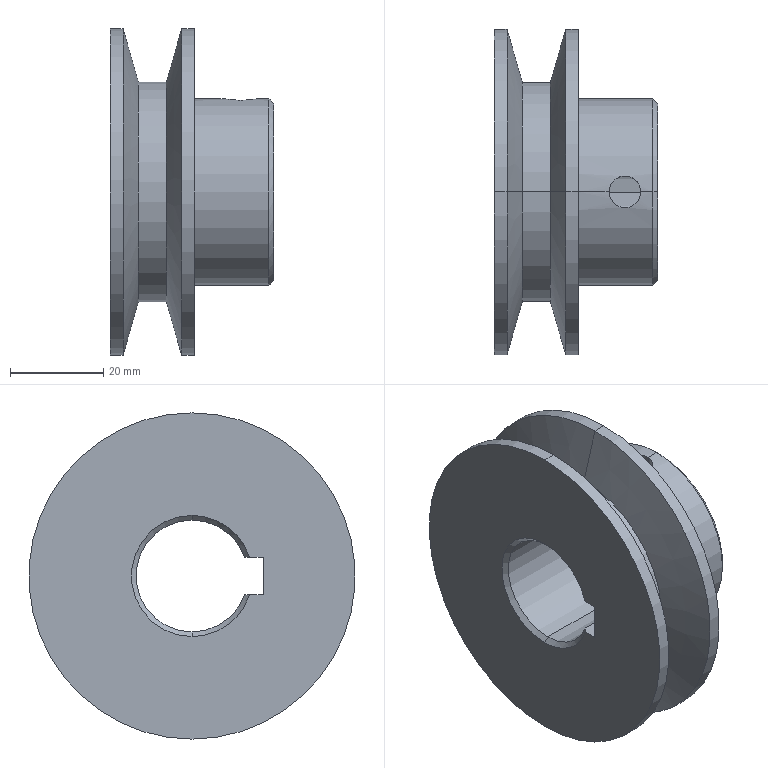Part | SolidWorks | features BaseBody 1 | 1 solid | 31 faces | box 35 x 70 x 70 mm | volume 53366 mm3 | cylinder 13 | cone 12 | plane 6 | commonest cylinder face diameters 70 x4 24 x3 6.8 x2 40 x2 47.1 x2
STEP:
#1=CARTESIAN_POINT('',(2.711,0.,35.));
#2=VERTEX_POINT('',#1);
#3=CARTESIAN_POINT('',(2.711,0.,-35.));
#4=VERTEX_POINT('',#3);
#5=CARTESIAN_POINT('',(2.711,0.,0.));
#6=DIRECTION('',(-1.,0.,0.));
#7=DIRECTION('',(0.,0.,1.));
#8=AXIS2_PLACEMENT_3D('',#5,#6,#7);
#9=CIRCLE('',#8,35.);
#10=EDGE_CURVE('',#2,#4,#9,.T.);
#11=ORIENTED_EDGE('',*,*,#10,.T.);
#12=CARTESIAN_POINT('',(0.,0.,-35.));
#13=VERTEX_POINT('',#12);
#14=CARTESIAN_POINT('',(0.,0.,-35.));
#15=DIRECTION('',(-1.,0.,0.));
#16=VECTOR('',#15,1000.);
#17=LINE('',#14,#16);
#18=EDGE_CURVE('',#4,#13,#17,.T.);
#19=ORIENTED_EDGE('',*,*,#18,.T.);
#20=CARTESIAN_POINT('',(0.,0.,35.));
#21=VERTEX_POINT('',#20);
#22=CARTESIAN_POINT('',(0.,0.,0.));
#23=DIRECTION('',(1.,0.,0.));
#24=DIRECTION('',(0.,0.,1.));
#25=AXIS2_PLACEMENT_3D('',#22,#23,#24);
#26=CIRCLE('',#25,35.);
#27=EDGE_CURVE('',#13,#21,#26,.T.);
#28=ORIENTED_EDGE('',*,*,#27,.T.);
#29=CARTESIAN_POINT('',(0.,0.,35.));
#30=DIRECTION('',(-1.,0.,0.));
#31=VECTOR('',#30,1000.);
#32=LINE('',#29,#31);
#33=EDGE_CURVE('',#2,#21,#32,.T.);
#34=ORIENTED_EDGE('',*,*,#33,.F.);
#35=EDGE_LOOP('',(#11,#19,#28,#34));
#36=FACE_OUTER_BOUND('',#35,.T.);
#37=CARTESIAN_POINT('',(0.,0.,0.));
#38=DIRECTION('',(-1.,0.,0.));
#39=DIRECTION('',(0.,0.,1.));
#40=AXIS2_PLACEMENT_3D('',#37,#38,#39);
#41=CYLINDRICAL_SURFACE('',#40,35.);
#42=ADVANCED_FACE('',(#36),#41,.T.);
#43=CARTESIAN_POINT('',(1.,0.,-12.));
#44=VERTEX_POINT('',#43);
#45=CARTESIAN_POINT('',(1.,-11.314,-4.));
#46=VERTEX_POINT('',#45);
#47=CARTESIAN_POINT('',(1.,0.,0.));
#48=DIRECTION('',(-1.,0.,0.));
#49=DIRECTION('',(0.,0.,1.));
#50=AXIS2_PLACEMENT_3D('',#47,#48,#49);
#51=CIRCLE('',#50,12.);
#52=EDGE_CURVE('',#44,#46,#51,.T.);
#53=ORIENTED_EDGE('',*,*,#52,.F.);
#54=CARTESIAN_POINT('',(0.,0.,-13.));
#55=VERTEX_POINT('',#54);
#56=CARTESIAN_POINT('',(0.,0.,-13.));
#57=DIRECTION('',(-0.7071,0.,-0.7071));
#58=VECTOR('',#57,1000.);
#59=LINE('',#56,#58);
#60=EDGE_CURVE('',#44,#55,#59,.T.);
#61=ORIENTED_EDGE('',*,*,#60,.T.);
#62=CARTESIAN_POINT('',(0.,-12.369,-4.));
#63=VERTEX_POINT('',#62);
#64=CARTESIAN_POINT('',(0.,0.,0.));
#65=DIRECTION('',(-1.,0.,0.));
#66=DIRECTION('',(0.,0.,1.));
#67=AXIS2_PLACEMENT_3D('',#64,#65,#66);
#68=CIRCLE('',#67,13.);
#69=EDGE_CURVE('',#55,#63,#68,.T.);
#70=ORIENTED_EDGE('',*,*,#69,.T.);
#71=CARTESIAN_POINT('',(1.,-11.314,-4.));
#72=CARTESIAN_POINT('',(0.6815,-11.652,-4.));
#73=CARTESIAN_POINT('',(0.3482,-12.003,-4.));
#74=CARTESIAN_POINT('',(0.,-12.369,-4.));
#75=B_SPLINE_CURVE_WITH_KNOTS('',3,(#71,#72,#73,#74),.UNSPECIFIED.,.F.,.F.,(4,4),(0.,1.),.UNSPECIFIED.);
#76=EDGE_CURVE('',#46,#63,#75,.T.);
#77=ORIENTED_EDGE('',*,*,#76,.F.);
#78=EDGE_LOOP('',(#53,#61,#70,#77));
#79=FACE_OUTER_BOUND('',#78,.T.);
#80=CARTESIAN_POINT('',(0.,0.,0.));
#81=DIRECTION('',(-1.,0.,0.));
#82=DIRECTION('',(0.,0.,1.));
#83=AXIS2_PLACEMENT_3D('',#80,#81,#82);
#84=CONICAL_SURFACE('',#83,13.,0.7854);
#85=ADVANCED_FACE('',(#79),#84,.F.);
#86=ORIENTED_EDGE('',*,*,#60,.F.);
#87=CARTESIAN_POINT('',(1.,0.,12.));
#88=VERTEX_POINT('',#87);
#89=CARTESIAN_POINT('',(1.,0.,0.));
#90=DIRECTION('',(-1.,0.,0.));
#91=DIRECTION('',(0.,0.,1.));
#92=AXIS2_PLACEMENT_3D('',#89,#90,#91);
#93=CIRCLE('',#92,12.);
#94=EDGE_CURVE('',#88,#44,#93,.T.);
#95=ORIENTED_EDGE('',*,*,#94,.F.);
#96=CARTESIAN_POINT('',(0.,0.,13.));
#97=VERTEX_POINT('',#96);
#98=CARTESIAN_POINT('',(0.,0.,13.));
#99=DIRECTION('',(-0.7071,0.,0.7071));
#100=VECTOR('',#99,1000.);
#101=LINE('',#98,#100);
#102=EDGE_CURVE('',#88,#97,#101,.T.);
#103=ORIENTED_EDGE('',*,*,#102,.T.);
#104=CARTESIAN_POINT('',(0.,0.,0.));
#105=DIRECTION('',(-1.,0.,0.));
#106=DIRECTION('',(0.,0.,1.));
#107=AXIS2_PLACEMENT_3D('',#104,#105,#106);
#108=CIRCLE('',#107,13.);
#109=EDGE_CURVE('',#97,#55,#108,.T.);
#110=ORIENTED_EDGE('',*,*,#109,.T.);
#111=EDGE_LOOP('',(#86,#95,#103,#110));
#112=FACE_OUTER_BOUND('',#111,.T.);
#113=CARTESIAN_POINT('',(0.,0.,0.));
#114=DIRECTION('',(-1.,0.,0.));
#115=DIRECTION('',(0.,0.,1.));
#116=AXIS2_PLACEMENT_3D('',#113,#114,#115);
#117=CONICAL_SURFACE('',#116,13.,0.7854);
#118=ADVANCED_FACE('',(#112),#117,.F.);
#119=CARTESIAN_POINT('',(5.995,0.,23.55));
#120=VERTEX_POINT('',#119);
#121=CARTESIAN_POINT('',(5.995,0.,-23.55));
#122=VERTEX_POINT('',#121);
#123=CARTESIAN_POINT('',(5.995,0.,0.));
#124=DIRECTION('',(-1.,0.,0.));
#125=DIRECTION('',(0.,0.,1.));
#126=AXIS2_PLACEMENT_3D('',#123,#124,#125);
#127=CIRCLE('',#126,23.55);
#128=EDGE_CURVE('',#120,#122,#127,.T.);
#129=ORIENTED_EDGE('',*,*,#128,.T.);
#130=CARTESIAN_POINT('',(2.711,0.,-35.));
#131=DIRECTION('',(-0.2756,0.,-0.9613));
#132=VECTOR('',#131,1000.);
#133=LINE('',#130,#132);
#134=EDGE_CURVE('',#122,#4,#133,.T.);
#135=ORIENTED_EDGE('',*,*,#134,.T.);
#136=ORIENTED_EDGE('',*,*,#10,.F.);
#137=CARTESIAN_POINT('',(2.711,0.,35.));
#138=DIRECTION('',(-0.2756,0.,0.9613));
#139=VECTOR('',#138,1000.);
#140=LINE('',#137,#139);
#141=EDGE_CURVE('',#120,#2,#140,.T.);
#142=ORIENTED_EDGE('',*,*,#141,.F.);
#143=EDGE_LOOP('',(#129,#135,#136,#142));
#144=FACE_OUTER_BOUND('',#143,.T.);
#145=CARTESIAN_POINT('',(2.711,0.,0.));
#146=DIRECTION('',(-1.,0.,0.));
#147=DIRECTION('',(0.,0.,1.));
#148=AXIS2_PLACEMENT_3D('',#145,#146,#147);
#149=CONICAL_SURFACE('',#148,35.,1.292);
#150=ADVANCED_FACE('',(#144),#149,.T.);
#151=CARTESIAN_POINT('',(34.,0.,-12.));
#152=VERTEX_POINT('',#151);
#153=CARTESIAN_POINT('',(34.,-11.314,-4.));
#154=VERTEX_POINT('',#153);
#155=CARTESIAN_POINT('',(34.,0.,0.));
#156=DIRECTION('',(-1.,0.,0.));
#157=DIRECTION('',(0.,0.,1.));
#158=AXIS2_PLACEMENT_3D('',#155,#156,#157);
#159=CIRCLE('',#158,12.);
#160=EDGE_CURVE('',#152,#154,#159,.T.);
#161=ORIENTED_EDGE('',*,*,#160,.F.);
#162=CARTESIAN_POINT('',(0.,0.,-12.));
#163=DIRECTION('',(-1.,0.,0.));
#164=VECTOR('',#163,1000.);
#165=LINE('',#162,#164);
#166=EDGE_CURVE('',#152,#44,#165,.T.);
#167=ORIENTED_EDGE('',*,*,#166,.T.);
#168=ORIENTED_EDGE('',*,*,#52,.T.);
#169=CARTESIAN_POINT('',(44.,-11.314,-4.));
#170=DIRECTION('',(1.,0.,0.));
#171=VECTOR('',#170,1000.);
#172=LINE('',#169,#171);
#173=EDGE_CURVE('',#46,#154,#172,.T.);
#174=ORIENTED_EDGE('',*,*,#173,.T.);
#175=EDGE_LOOP('',(#161,#167,#168,#174));
#176=FACE_OUTER_BOUND('',#175,.T.);
#177=CARTESIAN_POINT('',(0.,0.,0.));
#178=DIRECTION('',(-1.,0.,0.));
#179=DIRECTION('',(0.,0.,1.));
#180=AXIS2_PLACEMENT_3D('',#177,#178,#179);
#181=CYLINDRICAL_SURFACE('',#180,12.);
#182=ADVANCED_FACE('',(#176),#181,.F.);
#183=ORIENTED_EDGE('',*,*,#166,.F.);
#184=CARTESIAN_POINT('',(34.,0.,12.));
#185=VERTEX_POINT('',#184);
#186=CARTESIAN_POINT('',(34.,0.,0.));
#187=DIRECTION('',(-1.,0.,0.));
#188=DIRECTION('',(0.,0.,1.));
#189=AXIS2_PLACEMENT_3D('',#186,#187,#188);
#190=CIRCLE('',#189,12.);
#191=EDGE_CURVE('',#185,#152,#190,.T.);
#192=ORIENTED_EDGE('',*,*,#191,.F.);
#193=CARTESIAN_POINT('',(31.4,0.,12.));
#194=VERTEX_POINT('',#193);
#195=CARTESIAN_POINT('',(0.,0.,12.));
#196=DIRECTION('',(-1.,0.,0.));
#197=VECTOR('',#196,1000.);
#198=LINE('',#195,#197);
#199=EDGE_CURVE('',#185,#194,#198,.T.);
#200=ORIENTED_EDGE('',*,*,#199,.T.);
#201=CARTESIAN_POINT('',(24.6,0.,12.));
#202=VERTEX_POINT('',#201);
#203=CARTESIAN_POINT('',(24.6,0.,12.));
#204=CARTESIAN_POINT('',(24.6,0.2258,12.));
#205=CARTESIAN_POINT('',(24.622,0.4476,11.994));
#206=CARTESIAN_POINT('',(24.709,0.8837,11.969));
#207=CARTESIAN_POINT('',(24.775,1.1,11.951));
#208=CARTESIAN_POINT('',(24.946,1.511,11.906));
#209=CARTESIAN_POINT('',(25.051,1.706,11.88));
#210=CARTESIAN_POINT('',(25.297,2.075,11.821));
#211=CARTESIAN_POINT('',(25.44,2.248,11.789));
#212=CARTESIAN_POINT('',(25.752,2.56,11.725));
#213=CARTESIAN_POINT('',(25.922,2.701,11.693));
#214=CARTESIAN_POINT('',(26.293,2.949,11.633));
#215=CARTESIAN_POINT('',(26.489,3.054,11.605));
#216=CARTESIAN_POINT('',(26.898,3.224,11.559));
#217=CARTESIAN_POINT('',(27.113,3.29,11.54));
#218=CARTESIAN_POINT('',(27.552,3.378,11.515));
#219=CARTESIAN_POINT('',(27.774,3.4,11.508));
#220=CARTESIAN_POINT('',(28.22,3.4,11.508));
#221=CARTESIAN_POINT('',(28.446,3.378,11.515));
#222=CARTESIAN_POINT('',(28.883,3.291,11.54));
#223=CARTESIAN_POINT('',(29.096,3.226,11.558));
#224=CARTESIAN_POINT('',(29.509,3.055,11.605));
#225=CARTESIAN_POINT('',(29.706,2.949,11.633));
#226=CARTESIAN_POINT('',(30.073,2.704,11.692));
#227=CARTESIAN_POINT('',(30.246,2.562,11.724));
#228=CARTESIAN_POINT('',(30.56,2.248,11.789));
#229=CARTESIAN_POINT('',(30.7,2.078,11.82));
#230=CARTESIAN_POINT('',(30.946,1.711,11.879));
#231=CARTESIAN_POINT('',(31.053,1.512,11.906));
#232=CARTESIAN_POINT('',(31.224,1.102,11.951));
#233=CARTESIAN_POINT('',(31.289,0.8902,11.969));
#234=CARTESIAN_POINT('',(31.377,0.4517,11.994));
#235=CARTESIAN_POINT('',(31.4,0.2258,12.));
#236=CARTESIAN_POINT('',(31.4,0.,12.));
#237=B_SPLINE_CURVE_WITH_KNOTS('',3,(#203,#204,#205,#206,#207,#208,#209,#210,#211,#212,#213,#214,#215,#216,#217,#218,#219,#220,#221,#222,#223,#224,#225,#226,#227,#228,#229,#230,#231,#232,#233,#234,#235,#236),.UNSPECIFIED.,.F.,.F.,(4,2,2,2,2,2,2,2,2,2,2,2,2,2,2,2,4),(0.,0.0006676,0.001335,0.002003,0.00267,0.003338,0.004006,0.004673,0.005341,0.006008,0.006676,0.007343,0.008011,0.008679,0.009346,0.01001,0.01068),.UNSPECIFIED.);
#238=EDGE_CURVE('',#202,#194,#237,.T.);
#239=ORIENTED_EDGE('',*,*,#238,.F.);
#240=CARTESIAN_POINT('',(0.,0.,12.));
#241=DIRECTION('',(-1.,0.,0.));
#242=VECTOR('',#241,1000.);
#243=LINE('',#240,#242);
#244=EDGE_CURVE('',#202,#88,#243,.T.);
#245=ORIENTED_EDGE('',*,*,#244,.T.);
#246=ORIENTED_EDGE('',*,*,#94,.T.);
#247=EDGE_LOOP('',(#183,#192,#200,#239,#245,#246));
#248=FACE_OUTER_BOUND('',#247,.T.);
#249=CARTESIAN_POINT('',(0.,0.,0.));
#250=DIRECTION('',(-1.,0.,0.));
#251=DIRECTION('',(0.,0.,1.));
#252=AXIS2_PLACEMENT_3D('',#249,#250,#251);
#253=CYLINDRICAL_SURFACE('',#252,12.);
#254=ADVANCED_FACE('',(#248),#253,.F.);
#255=CARTESIAN_POINT('',(12.005,0.,23.55));
#256=VERTEX_POINT('',#255);
#257=CARTESIAN_POINT('',(12.005,0.,-23.55));
#258=VERTEX_POINT('',#257);
#259=CARTESIAN_POINT('',(12.005,0.,0.));
#260=DIRECTION('',(-1.,0.,0.));
#261=DIRECTION('',(0.,0.,1.));
#262=AXIS2_PLACEMENT_3D('',#259,#260,#261);
#263=CIRCLE('',#262,23.55);
#264=EDGE_CURVE('',#256,#258,#263,.T.);
#265=ORIENTED_EDGE('',*,*,#264,.T.);
#266=CARTESIAN_POINT('',(0.,0.,-23.55));
#267=DIRECTION('',(-1.,0.,0.));
#268=VECTOR('',#267,1000.);
#269=LINE('',#266,#268);
#270=EDGE_CURVE('',#258,#122,#269,.T.);
#271=ORIENTED_EDGE('',*,*,#270,.T.);
#272=ORIENTED_EDGE('',*,*,#128,.F.);
#273=CARTESIAN_POINT('',(0.,0.,23.55));
#274=DIRECTION('',(-1.,0.,0.));
#275=VECTOR('',#274,1000.);
#276=LINE('',#273,#275);
#277=EDGE_CURVE('',#256,#120,#276,.T.);
#278=ORIENTED_EDGE('',*,*,#277,.F.);
#279=EDGE_LOOP('',(#265,#271,#272,#278));
#280=FACE_OUTER_BOUND('',#279,.T.);
#281=CARTESIAN_POINT('',(0.,0.,0.));
#282=DIRECTION('',(-1.,0.,0.));
#283=DIRECTION('',(0.,0.,1.));
#284=AXIS2_PLACEMENT_3D('',#281,#282,#283);
#285=CYLINDRICAL_SURFACE('',#284,23.55);
#286=ADVANCED_FACE('',(#280),#285,.T.);
#287=CARTESIAN_POINT('',(34.,-11.314,4.));
#288=VERTEX_POINT('',#287);
#289=CARTESIAN_POINT('',(34.,0.,0.));
#290=DIRECTION('',(-1.,0.,0.));
#291=DIRECTION('',(0.,0.,1.));
#292=AXIS2_PLACEMENT_3D('',#289,#290,#291);
#293=CIRCLE('',#292,12.);
#294=EDGE_CURVE('',#288,#185,#293,.T.);
#295=ORIENTED_EDGE('',*,*,#294,.T.);
#296=CARTESIAN_POINT('',(35.,0.,13.));
#297=VERTEX_POINT('',#296);
#298=CARTESIAN_POINT('',(35.,0.,13.));
#299=DIRECTION('',(0.7071,0.,0.7071));
#300=VECTOR('',#299,1000.);
#301=LINE('',#298,#300);
#302=EDGE_CURVE('',#185,#297,#301,.T.);
#303=ORIENTED_EDGE('',*,*,#302,.T.);
#304=CARTESIAN_POINT('',(35.,-12.369,4.));
#305=VERTEX_POINT('',#304);
#306=CARTESIAN_POINT('',(35.,0.,0.));
#307=DIRECTION('',(1.,0.,0.));
#308=DIRECTION('',(0.,0.,-1.));
#309=AXIS2_PLACEMENT_3D('',#306,#307,#308);
#310=CIRCLE('',#309,13.);
#311=EDGE_CURVE('',#297,#305,#310,.T.);
#312=ORIENTED_EDGE('',*,*,#311,.T.);
#313=CARTESIAN_POINT('',(34.,-11.314,4.));
#314=CARTESIAN_POINT('',(34.318,-11.652,4.));
#315=CARTESIAN_POINT('',(34.652,-12.003,4.));
#316=CARTESIAN_POINT('',(35.,-12.369,4.));
#317=B_SPLINE_CURVE_WITH_KNOTS('',3,(#313,#314,#315,#316),.UNSPECIFIED.,.F.,.F.,(4,4),(0.,1.),.UNSPECIFIED.);
#318=EDGE_CURVE('',#288,#305,#317,.T.);
#319=ORIENTED_EDGE('',*,*,#318,.F.);
#320=EDGE_LOOP('',(#295,#303,#312,#319));
#321=FACE_OUTER_BOUND('',#320,.T.);
#322=CARTESIAN_POINT('',(35.,0.,0.));
#323=DIRECTION('',(1.,0.,0.));
#324=DIRECTION('',(0.,0.,-1.));
#325=AXIS2_PLACEMENT_3D('',#322,#323,#324);
#326=CONICAL_SURFACE('',#325,13.,0.7854);
#327=ADVANCED_FACE('',(#321),#326,.F.);
#328=ORIENTED_EDGE('',*,*,#302,.F.);
#329=ORIENTED_EDGE('',*,*,#191,.T.);
#330=CARTESIAN_POINT('',(35.,0.,-13.));
#331=VERTEX_POINT('',#330);
#332=CARTESIAN_POINT('',(35.,0.,-13.));
#333=DIRECTION('',(0.7071,0.,-0.7071));
#334=VECTOR('',#333,1000.);
#335=LINE('',#332,#334);
#336=EDGE_CURVE('',#152,#331,#335,.T.);
#337=ORIENTED_EDGE('',*,*,#336,.T.);
#338=CARTESIAN_POINT('',(35.,0.,0.));
#339=DIRECTION('',(1.,0.,0.));
#340=DIRECTION('',(0.,0.,-1.));
#341=AXIS2_PLACEMENT_3D('',#338,#339,#340);
#342=CIRCLE('',#341,13.);
#343=EDGE_CURVE('',#331,#297,#342,.T.);
#344=ORIENTED_EDGE('',*,*,#343,.T.);
#345=EDGE_LOOP('',(#328,#329,#337,#344));
#346=FACE_OUTER_BOUND('',#345,.T.);
#347=CARTESIAN_POINT('',(35.,0.,0.));
#348=DIRECTION('',(1.,0.,0.));
#349=DIRECTION('',(0.,0.,-1.));
#350=AXIS2_PLACEMENT_3D('',#347,#348,#349);
#351=CONICAL_SURFACE('',#350,13.,0.7854);
#352=ADVANCED_FACE('',(#346),#351,.F.);
#353=CARTESIAN_POINT('',(31.4,0.,20.));
#354=VERTEX_POINT('',#353);
#355=CARTESIAN_POINT('',(24.6,0.,20.));
#356=VERTEX_POINT('',#355);
#357=CARTESIAN_POINT('',(31.4,0.,20.));
#358=CARTESIAN_POINT('',(31.4,-0.225,20.));
#359=CARTESIAN_POINT('',(31.378,-0.4462,19.996));
#360=CARTESIAN_POINT('',(31.291,-0.8813,19.982));
#361=CARTESIAN_POINT('',(31.226,-1.097,19.971));
#362=CARTESIAN_POINT('',(31.055,-1.509,19.944));
#363=CARTESIAN_POINT('',(30.951,-1.704,19.928));
#364=CARTESIAN_POINT('',(30.704,-2.073,19.893));
#365=CARTESIAN_POINT('',(30.561,-2.248,19.874));
#366=CARTESIAN_POINT('',(30.248,-2.561,19.836));
#367=CARTESIAN_POINT('',(30.077,-2.701,19.817));
#368=CARTESIAN_POINT('',(29.705,-2.95,19.782));
#369=CARTESIAN_POINT('',(29.508,-3.055,19.765));
#370=CARTESIAN_POINT('',(29.099,-3.225,19.738));
#371=CARTESIAN_POINT('',(28.885,-3.291,19.728));
#372=CARTESIAN_POINT('',(28.446,-3.378,19.713));
#373=CARTESIAN_POINT('',(28.225,-3.4,19.709));
#374=CARTESIAN_POINT('',(27.78,-3.4,19.709));
#375=CARTESIAN_POINT('',(27.555,-3.378,19.713));
#376=CARTESIAN_POINT('',(27.118,-3.291,19.727));
#377=CARTESIAN_POINT('',(26.906,-3.227,19.738));
#378=CARTESIAN_POINT('',(26.494,-3.057,19.765));
#379=CARTESIAN_POINT('',(26.296,-2.95,19.782));
#380=CARTESIAN_POINT('',(25.928,-2.705,19.817));
#381=CARTESIAN_POINT('',(25.756,-2.564,19.836));
#382=CARTESIAN_POINT('',(25.439,-2.247,19.874));
#383=CARTESIAN_POINT('',(25.298,-2.076,19.893));
#384=CARTESIAN_POINT('',(25.052,-1.709,19.928));
#385=CARTESIAN_POINT('',(24.945,-1.51,19.944));
#386=CARTESIAN_POINT('',(24.775,-1.099,19.971));
#387=CARTESIAN_POINT('',(24.71,-0.8867,19.982));
#388=CARTESIAN_POINT('',(24.623,-0.4503,19.996));
#389=CARTESIAN_POINT('',(24.6,-0.225,20.));
#390=CARTESIAN_POINT('',(24.6,0.,20.));
#391=B_SPLINE_CURVE_WITH_KNOTS('',3,(#357,#358,#359,#360,#361,#362,#363,#364,#365,#366,#367,#368,#369,#370,#371,#372,#373,#374,#375,#376,#377,#378,#379,#380,#381,#382,#383,#384,#385,#386,#387,#388,#389,#390),.UNSPECIFIED.,.F.,.F.,(4,2,2,2,2,2,2,2,2,2,2,2,2,2,2,2,4),(0.01065,0.01131,0.01198,0.01264,0.01331,0.01397,0.01464,0.0153,0.01597,0.01664,0.0173,0.01797,0.01863,0.0193,0.01996,0.02063,0.02129),.UNSPECIFIED.);
#392=EDGE_CURVE('',#354,#356,#391,.T.);
#393=ORIENTED_EDGE('',*,*,#392,.F.);
#394=CARTESIAN_POINT('',(31.4,0.,0.));
#395=DIRECTION('',(0.,0.,-1.));
#396=VECTOR('',#395,1000.);
#397=LINE('',#394,#396);
#398=EDGE_CURVE('',#354,#194,#397,.T.);
#399=ORIENTED_EDGE('',*,*,#398,.T.);
#400=CARTESIAN_POINT('',(31.4,0.,12.));
#401=CARTESIAN_POINT('',(31.4,-0.2258,12.));
#402=CARTESIAN_POINT('',(31.378,-0.4476,11.994));
#403=CARTESIAN_POINT('',(31.291,-0.8837,11.969));
#404=CARTESIAN_POINT('',(31.225,-1.1,11.951));
#405=CARTESIAN_POINT('',(31.054,-1.511,11.906));
#406=CARTESIAN_POINT('',(30.949,-1.706,11.88));
#407=CARTESIAN_POINT('',(30.703,-2.075,11.821));
#408=CARTESIAN_POINT('',(30.56,-2.248,11.789));
#409=CARTESIAN_POINT('',(30.248,-2.56,11.725));
#410=CARTESIAN_POINT('',(30.078,-2.701,11.693));
#411=CARTESIAN_POINT('',(29.707,-2.949,11.633));
#412=CARTESIAN_POINT('',(29.511,-3.054,11.605));
#413=CARTESIAN_POINT('',(29.102,-3.224,11.559));
#414=CARTESIAN_POINT('',(28.887,-3.29,11.54));
#415=CARTESIAN_POINT('',(28.448,-3.378,11.515));
#416=CARTESIAN_POINT('',(28.226,-3.4,11.508));
#417=CARTESIAN_POINT('',(27.78,-3.4,11.508));
#418=CARTESIAN_POINT('',(27.554,-3.378,11.515));
#419=CARTESIAN_POINT('',(27.117,-3.291,11.54));
#420=CARTESIAN_POINT('',(26.904,-3.226,11.558));
#421=CARTESIAN_POINT('',(26.491,-3.055,11.605));
#422=CARTESIAN_POINT('',(26.294,-2.949,11.633));
#423=CARTESIAN_POINT('',(25.927,-2.704,11.692));
#424=CARTESIAN_POINT('',(25.754,-2.562,11.724));
#425=CARTESIAN_POINT('',(25.44,-2.248,11.789));
#426=CARTESIAN_POINT('',(25.3,-2.078,11.82));
#427=CARTESIAN_POINT('',(25.054,-1.711,11.879));
#428=CARTESIAN_POINT('',(24.947,-1.512,11.906));
#429=CARTESIAN_POINT('',(24.776,-1.102,11.951));
#430=CARTESIAN_POINT('',(24.711,-0.8902,11.969));
#431=CARTESIAN_POINT('',(24.623,-0.4517,11.994));
#432=CARTESIAN_POINT('',(24.6,-0.2258,12.));
#433=CARTESIAN_POINT('',(24.6,0.,12.));
#434=B_SPLINE_CURVE_WITH_KNOTS('',3,(#400,#401,#402,#403,#404,#405,#406,#407,#408,#409,#410,#411,#412,#413,#414,#415,#416,#417,#418,#419,#420,#421,#422,#423,#424,#425,#426,#427,#428,#429,#430,#431,#432,#433),.UNSPECIFIED.,.F.,.F.,(4,2,2,2,2,2,2,2,2,2,2,2,2,2,2,2,4),(0.01068,0.01135,0.01202,0.01268,0.01335,0.01402,0.01469,0.01535,0.01602,0.01669,0.01736,0.01802,0.01869,0.01936,0.02003,0.02069,0.02136),.UNSPECIFIED.);
#435=EDGE_CURVE('',#194,#202,#434,.T.);
#436=ORIENTED_EDGE('',*,*,#435,.T.);
#437=CARTESIAN_POINT('',(24.6,0.,0.));
#438=DIRECTION('',(0.,0.,-1.));
#439=VECTOR('',#438,1000.);
#440=LINE('',#437,#439);
#441=EDGE_CURVE('',#356,#202,#440,.T.);
#442=ORIENTED_EDGE('',*,*,#441,.F.);
#443=EDGE_LOOP('',(#393,#399,#436,#442));
#444=FACE_OUTER_BOUND('',#443,.T.);
#445=CARTESIAN_POINT('',(28.,0.,0.));
#446=DIRECTION('',(0.,0.,-1.));
#447=DIRECTION('',(-1.,0.,0.));
#448=AXIS2_PLACEMENT_3D('',#445,#446,#447);
#449=CYLINDRICAL_SURFACE('',#448,3.4);
#450=ADVANCED_FACE('',(#444),#449,.F.);
#451=CARTESIAN_POINT('',(35.,0.,19.));
#452=VERTEX_POINT('',#451);
#453=CARTESIAN_POINT('',(35.,0.,-19.));
#454=VERTEX_POINT('',#453);
#455=CARTESIAN_POINT('',(35.,0.,0.));
#456=DIRECTION('',(-1.,0.,0.));
#457=DIRECTION('',(0.,0.,1.));
#458=AXIS2_PLACEMENT_3D('',#455,#456,#457);
#459=CIRCLE('',#458,19.);
#460=EDGE_CURVE('',#452,#454,#459,.T.);
#461=ORIENTED_EDGE('',*,*,#460,.T.);
#462=CARTESIAN_POINT('',(34.,0.,-20.));
#463=VERTEX_POINT('',#462);
#464=CARTESIAN_POINT('',(34.,0.,-20.));
#465=DIRECTION('',(-0.7071,0.,-0.7071));
#466=VECTOR('',#465,1000.);
#467=LINE('',#464,#466);
#468=EDGE_CURVE('',#454,#463,#467,.T.);
#469=ORIENTED_EDGE('',*,*,#468,.T.);
#470=CARTESIAN_POINT('',(34.,0.,20.));
#471=VERTEX_POINT('',#470);
#472=CARTESIAN_POINT('',(34.,0.,0.));
#473=DIRECTION('',(1.,0.,0.));
#474=DIRECTION('',(0.,0.,1.));
#475=AXIS2_PLACEMENT_3D('',#472,#473,#474);
#476=CIRCLE('',#475,20.);
#477=EDGE_CURVE('',#463,#471,#476,.T.);
#478=ORIENTED_EDGE('',*,*,#477,.T.);
#479=CARTESIAN_POINT('',(34.,0.,20.));
#480=DIRECTION('',(-0.7071,0.,0.7071));
#481=VECTOR('',#480,1000.);
#482=LINE('',#479,#481);
#483=EDGE_CURVE('',#452,#471,#482,.T.);
#484=ORIENTED_EDGE('',*,*,#483,.F.);
#485=EDGE_LOOP('',(#461,#469,#478,#484));
#486=FACE_OUTER_BOUND('',#485,.T.);
#487=CARTESIAN_POINT('',(34.,0.,0.));
#488=DIRECTION('',(-1.,0.,0.));
#489=DIRECTION('',(0.,0.,1.));
#490=AXIS2_PLACEMENT_3D('',#487,#488,#489);
#491=CONICAL_SURFACE('',#490,20.,0.7854);
#492=ADVANCED_FACE('',(#486),#491,.T.);
#493=ORIENTED_EDGE('',*,*,#264,.F.);
#494=CARTESIAN_POINT('',(15.289,0.,35.));
#495=VERTEX_POINT('',#494);
#496=CARTESIAN_POINT('',(15.289,0.,35.));
#497=DIRECTION('',(0.2756,0.,0.9613));
#498=VECTOR('',#497,1000.);
#499=LINE('',#496,#498);
#500=EDGE_CURVE('',#256,#495,#499,.T.);
#501=ORIENTED_EDGE('',*,*,#500,.T.);
#502=CARTESIAN_POINT('',(15.289,0.,-35.));
#503=VERTEX_POINT('',#502);
#504=CARTESIAN_POINT('',(15.289,0.,0.));
#505=DIRECTION('',(-1.,0.,0.));
#506=DIRECTION('',(0.,0.,-1.));
#507=AXIS2_PLACEMENT_3D('',#504,#505,#506);
#508=CIRCLE('',#507,35.);
#509=EDGE_CURVE('',#495,#503,#508,.T.);
#510=ORIENTED_EDGE('',*,*,#509,.T.);
#511=CARTESIAN_POINT('',(15.289,0.,-35.));
#512=DIRECTION('',(0.2756,0.,-0.9613));
#513=VECTOR('',#512,1000.);
#514=LINE('',#511,#513);
#515=EDGE_CURVE('',#258,#503,#514,.T.);
#516=ORIENTED_EDGE('',*,*,#515,.F.);
#517=EDGE_LOOP('',(#493,#501,#510,#516));
#518=FACE_OUTER_BOUND('',#517,.T.);
#519=CARTESIAN_POINT('',(15.289,0.,0.));
#520=DIRECTION('',(1.,0.,0.));
#521=DIRECTION('',(0.,0.,-1.));
#522=AXIS2_PLACEMENT_3D('',#519,#520,#521);
#523=CONICAL_SURFACE('',#522,35.,1.292);
#524=ADVANCED_FACE('',(#518),#523,.T.);
#525=ORIENTED_EDGE('',*,*,#477,.F.);
#526=CARTESIAN_POINT('',(18.,0.,-20.));
#527=VERTEX_POINT('',#526);
#528=CARTESIAN_POINT('',(0.,0.,-20.));
#529=DIRECTION('',(-1.,0.,0.));
#530=VECTOR('',#529,1000.);
#531=LINE('',#528,#530);
#532=EDGE_CURVE('',#463,#527,#531,.T.);
#533=ORIENTED_EDGE('',*,*,#532,.T.);
#534=CARTESIAN_POINT('',(18.,0.,20.));
#535=VERTEX_POINT('',#534);
#536=CARTESIAN_POINT('',(18.,0.,0.));
#537=DIRECTION('',(1.,0.,0.));
#538=DIRECTION('',(0.,0.,1.));
#539=AXIS2_PLACEMENT_3D('',#536,#537,#538);
#540=CIRCLE('',#539,20.);
#541=EDGE_CURVE('',#527,#535,#540,.T.);
#542=ORIENTED_EDGE('',*,*,#541,.T.);
#543=CARTESIAN_POINT('',(0.,0.,20.));
#544=DIRECTION('',(-1.,0.,0.));
#545=VECTOR('',#544,1000.);
#546=LINE('',#543,#545);
#547=EDGE_CURVE('',#356,#535,#546,.T.);
#548=ORIENTED_EDGE('',*,*,#547,.F.);
#549=CARTESIAN_POINT('',(24.6,0.,20.));
#550=CARTESIAN_POINT('',(24.6,0.225,20.));
#551=CARTESIAN_POINT('',(24.622,0.4462,19.996));
#552=CARTESIAN_POINT('',(24.709,0.8813,19.982));
#553=CARTESIAN_POINT('',(24.774,1.097,19.971));
#554=CARTESIAN_POINT('',(24.945,1.509,19.944));
#555=CARTESIAN_POINT('',(25.049,1.704,19.928));
#556=CARTESIAN_POINT('',(25.296,2.073,19.893));
#557=CARTESIAN_POINT('',(25.439,2.248,19.874));
#558=CARTESIAN_POINT('',(25.752,2.561,19.836));
#559=CARTESIAN_POINT('',(25.923,2.701,19.817));
#560=CARTESIAN_POINT('',(26.295,2.95,19.782));
#561=CARTESIAN_POINT('',(26.492,3.055,19.765));
#562=CARTESIAN_POINT('',(26.901,3.225,19.738));
#563=CARTESIAN_POINT('',(27.115,3.291,19.728));
#564=CARTESIAN_POINT('',(27.554,3.378,19.713));
#565=CARTESIAN_POINT('',(27.775,3.4,19.709));
#566=CARTESIAN_POINT('',(28.22,3.4,19.709));
#567=CARTESIAN_POINT('',(28.445,3.378,19.713));
#568=CARTESIAN_POINT('',(28.882,3.291,19.727));
#569=CARTESIAN_POINT('',(29.094,3.227,19.738));
#570=CARTESIAN_POINT('',(29.506,3.057,19.765));
#571=CARTESIAN_POINT('',(29.704,2.95,19.782));
#572=CARTESIAN_POINT('',(30.072,2.705,19.817));
#573=CARTESIAN_POINT('',(30.244,2.564,19.836));
#574=CARTESIAN_POINT('',(30.561,2.247,19.874));
#575=CARTESIAN_POINT('',(30.702,2.076,19.893));
#576=CARTESIAN_POINT('',(30.948,1.709,19.928));
#577=CARTESIAN_POINT('',(31.055,1.51,19.944));
#578=CARTESIAN_POINT('',(31.225,1.099,19.971));
#579=CARTESIAN_POINT('',(31.29,0.8867,19.982));
#580=CARTESIAN_POINT('',(31.377,0.4503,19.996));
#581=CARTESIAN_POINT('',(31.4,0.225,20.));
#582=CARTESIAN_POINT('',(31.4,0.,20.));
#583=B_SPLINE_CURVE_WITH_KNOTS('',3,(#549,#550,#551,#552,#553,#554,#555,#556,#557,#558,#559,#560,#561,#562,#563,#564,#565,#566,#567,#568,#569,#570,#571,#572,#573,#574,#575,#576,#577,#578,#579,#580,#581,#582),.UNSPECIFIED.,.F.,.F.,(4,2,2,2,2,2,2,2,2,2,2,2,2,2,2,2,4),(0.,0.0006654,0.001331,0.001996,0.002662,0.003327,0.003992,0.004658,0.005323,0.005989,0.006654,0.00732,0.007985,0.00865,0.009316,0.009981,0.01065),.UNSPECIFIED.);
#584=EDGE_CURVE('',#356,#354,#583,.T.);
#585=ORIENTED_EDGE('',*,*,#584,.T.);
#586=CARTESIAN_POINT('',(0.,0.,20.));
#587=DIRECTION('',(-1.,0.,0.));
#588=VECTOR('',#587,1000.);
#589=LINE('',#586,#588);
#590=EDGE_CURVE('',#471,#354,#589,.T.);
#591=ORIENTED_EDGE('',*,*,#590,.F.);
#592=EDGE_LOOP('',(#525,#533,#542,#548,#585,#591));
#593=FACE_OUTER_BOUND('',#592,.T.);
#594=CARTESIAN_POINT('',(0.,0.,0.));
#595=DIRECTION('',(-1.,0.,0.));
#596=DIRECTION('',(0.,0.,1.));
#597=AXIS2_PLACEMENT_3D('',#594,#595,#596);
#598=CYLINDRICAL_SURFACE('',#597,20.);
#599=ADVANCED_FACE('',(#593),#598,.T.);
#600=CARTESIAN_POINT('',(18.,0.,35.));
#601=VERTEX_POINT('',#600);
#602=CARTESIAN_POINT('',(18.,0.,-35.));
#603=VERTEX_POINT('',#602);
#604=CARTESIAN_POINT('',(18.,0.,0.));
#605=DIRECTION('',(-1.,0.,0.));
#606=DIRECTION('',(0.,0.,1.));
#607=AXIS2_PLACEMENT_3D('',#604,#605,#606);
#608=CIRCLE('',#607,35.);
#609=EDGE_CURVE('',#601,#603,#608,.T.);
#610=ORIENTED_EDGE('',*,*,#609,.T.);
#611=CARTESIAN_POINT('',(0.,0.,-35.));
#612=DIRECTION('',(-1.,0.,0.));
#613=VECTOR('',#612,1000.);
#614=LINE('',#611,#613);
#615=EDGE_CURVE('',#603,#503,#614,.T.);
#616=ORIENTED_EDGE('',*,*,#615,.T.);
#617=ORIENTED_EDGE('',*,*,#509,.F.);
#618=CARTESIAN_POINT('',(0.,0.,35.));
#619=DIRECTION('',(-1.,0.,0.));
#620=VECTOR('',#619,1000.);
#621=LINE('',#618,#620);
#622=EDGE_CURVE('',#601,#495,#621,.T.);
#623=ORIENTED_EDGE('',*,*,#622,.F.);
#624=EDGE_LOOP('',(#610,#616,#617,#623));
#625=FACE_OUTER_BOUND('',#624,.T.);
#626=CARTESIAN_POINT('',(0.,0.,0.));
#627=DIRECTION('',(-1.,0.,0.));
#628=DIRECTION('',(0.,0.,1.));
#629=AXIS2_PLACEMENT_3D('',#626,#627,#628);
#630=CYLINDRICAL_SURFACE('',#629,35.);
#631=ADVANCED_FACE('',(#625),#630,.T.);
#632=CARTESIAN_POINT('',(0.,0.,0.));
#633=DIRECTION('',(1.,0.,0.));
#634=DIRECTION('',(0.,0.,1.));
#635=AXIS2_PLACEMENT_3D('',#632,#633,#634);
#636=CIRCLE('',#635,35.);
#637=EDGE_CURVE('',#21,#13,#636,.T.);
#638=ORIENTED_EDGE('',*,*,#637,.F.);
#639=ORIENTED_EDGE('',*,*,#27,.F.);
#640=EDGE_LOOP('',(#638,#639));
#641=FACE_OUTER_BOUND('',#640,.T.);
#642=CARTESIAN_POINT('',(0.,-15.3,-4.));
#643=VERTEX_POINT('',#642);
#644=CARTESIAN_POINT('',(0.,12.,-4.));
#645=DIRECTION('',(0.,-1.,0.));
#646=VECTOR('',#645,1000.);
#647=LINE('',#644,#646);
#648=EDGE_CURVE('',#63,#643,#647,.T.);
#649=ORIENTED_EDGE('',*,*,#648,.F.);
#650=ORIENTED_EDGE('',*,*,#69,.F.);
#651=ORIENTED_EDGE('',*,*,#109,.F.);
#652=CARTESIAN_POINT('',(0.,-12.369,4.));
#653=VERTEX_POINT('',#652);
#654=CARTESIAN_POINT('',(0.,0.,0.));
#655=DIRECTION('',(-1.,0.,0.));
#656=DIRECTION('',(0.,0.,1.));
#657=AXIS2_PLACEMENT_3D('',#654,#655,#656);
#658=CIRCLE('',#657,13.);
#659=EDGE_CURVE('',#653,#97,#658,.T.);
#660=ORIENTED_EDGE('',*,*,#659,.F.);
#661=CARTESIAN_POINT('',(0.,-15.3,4.));
#662=VERTEX_POINT('',#661);
#663=CARTESIAN_POINT('',(0.,12.,4.));
#664=DIRECTION('',(0.,1.,0.));
#665=VECTOR('',#664,1000.);
#666=LINE('',#663,#665);
#667=EDGE_CURVE('',#662,#653,#666,.T.);
#668=ORIENTED_EDGE('',*,*,#667,.F.);
#669=CARTESIAN_POINT('',(0.,-15.3,0.));
#670=DIRECTION('',(0.,0.,1.));
#671=VECTOR('',#670,1000.);
#672=LINE('',#669,#671);
#673=EDGE_CURVE('',#643,#662,#672,.T.);
#674=ORIENTED_EDGE('',*,*,#673,.F.);
#675=EDGE_LOOP('',(#649,#650,#651,#660,#668,#674));
#676=FACE_BOUND('',#675,.T.);
#677=CARTESIAN_POINT('',(0.,12.,0.));
#678=DIRECTION('',(1.,0.,0.));
#679=DIRECTION('',(0.,0.,-1.));
#680=AXIS2_PLACEMENT_3D('',#677,#678,#679);
#681=PLANE('',#680);
#682=ADVANCED_FACE('',(#641,#676),#681,.F.);
#683=ORIENTED_EDGE('',*,*,#18,.F.);
#684=CARTESIAN_POINT('',(2.711,0.,0.));
#685=DIRECTION('',(-1.,0.,0.));
#686=DIRECTION('',(0.,0.,1.));
#687=AXIS2_PLACEMENT_3D('',#684,#685,#686);
#688=CIRCLE('',#687,35.);
#689=EDGE_CURVE('',#4,#2,#688,.T.);
#690=ORIENTED_EDGE('',*,*,#689,.T.);
#691=ORIENTED_EDGE('',*,*,#33,.T.);
#692=ORIENTED_EDGE('',*,*,#637,.T.);
#693=EDGE_LOOP('',(#683,#690,#691,#692));
#694=FACE_OUTER_BOUND('',#693,.T.);
#695=CARTESIAN_POINT('',(0.,0.,0.));
#696=DIRECTION('',(-1.,0.,0.));
#697=DIRECTION('',(0.,0.,1.));
#698=AXIS2_PLACEMENT_3D('',#695,#696,#697);
#699=CYLINDRICAL_SURFACE('',#698,35.);
#700=ADVANCED_FACE('',(#694),#699,.T.);
#701=ORIENTED_EDGE('',*,*,#102,.F.);
#702=CARTESIAN_POINT('',(1.,-11.314,4.));
#703=VERTEX_POINT('',#702);
#704=CARTESIAN_POINT('',(1.,0.,0.));
#705=DIRECTION('',(-1.,0.,0.));
#706=DIRECTION('',(0.,0.,1.));
#707=AXIS2_PLACEMENT_3D('',#704,#705,#706);
#708=CIRCLE('',#707,12.);
#709=EDGE_CURVE('',#703,#88,#708,.T.);
#710=ORIENTED_EDGE('',*,*,#709,.F.);
#711=CARTESIAN_POINT('',(0.,-12.369,4.));
#712=CARTESIAN_POINT('',(0.3482,-12.003,4.));
#713=CARTESIAN_POINT('',(0.6815,-11.652,4.));
#714=CARTESIAN_POINT('',(1.,-11.314,4.));
#715=B_SPLINE_CURVE_WITH_KNOTS('',3,(#711,#712,#713,#714),.UNSPECIFIED.,.F.,.F.,(4,4),(0.,1.),.UNSPECIFIED.);
#716=EDGE_CURVE('',#653,#703,#715,.T.);
#717=ORIENTED_EDGE('',*,*,#716,.F.);
#718=ORIENTED_EDGE('',*,*,#659,.T.);
#719=EDGE_LOOP('',(#701,#710,#717,#718));
#720=FACE_OUTER_BOUND('',#719,.T.);
#721=CARTESIAN_POINT('',(0.,0.,0.));
#722=DIRECTION('',(-1.,0.,0.));
#723=DIRECTION('',(0.,0.,1.));
#724=AXIS2_PLACEMENT_3D('',#721,#722,#723);
#725=CONICAL_SURFACE('',#724,13.,0.7854);
#726=ADVANCED_FACE('',(#720),#725,.F.);
#727=CARTESIAN_POINT('',(44.,-11.314,4.));
#728=DIRECTION('',(-1.,0.,0.));
#729=VECTOR('',#728,1000.);
#730=LINE('',#727,#729);
#731=EDGE_CURVE('',#288,#703,#730,.T.);
#732=ORIENTED_EDGE('',*,*,#731,.F.);
#733=ORIENTED_EDGE('',*,*,#318,.T.);
#734=CARTESIAN_POINT('',(35.,-15.3,4.));
#735=VERTEX_POINT('',#734);
#736=CARTESIAN_POINT('',(35.,-15.3,4.));
#737=DIRECTION('',(0.,1.,0.));
#738=VECTOR('',#737,1000.);
#739=LINE('',#736,#738);
#740=EDGE_CURVE('',#735,#305,#739,.T.);
#741=ORIENTED_EDGE('',*,*,#740,.F.);
#742=CARTESIAN_POINT('',(44.,-15.3,4.));
#743=DIRECTION('',(1.,0.,0.));
#744=VECTOR('',#743,1000.);
#745=LINE('',#742,#744);
#746=EDGE_CURVE('',#662,#735,#745,.T.);
#747=ORIENTED_EDGE('',*,*,#746,.F.);
#748=ORIENTED_EDGE('',*,*,#667,.T.);
#749=ORIENTED_EDGE('',*,*,#716,.T.);
#750=EDGE_LOOP('',(#732,#733,#741,#747,#748,#749));
#751=FACE_OUTER_BOUND('',#750,.T.);
#752=CARTESIAN_POINT('',(44.,-15.3,4.));
#753=DIRECTION('',(0.,0.,1.));
#754=DIRECTION('',(1.,0.,0.));
#755=AXIS2_PLACEMENT_3D('',#752,#753,#754);
#756=PLANE('',#755);
#757=ADVANCED_FACE('',(#751),#756,.F.);
#758=ORIENTED_EDGE('',*,*,#673,.T.);
#759=ORIENTED_EDGE('',*,*,#746,.T.);
#760=CARTESIAN_POINT('',(35.,-15.3,-4.));
#761=VERTEX_POINT('',#760);
#762=CARTESIAN_POINT('',(35.,-15.3,-4.));
#763=DIRECTION('',(0.,0.,1.));
#764=VECTOR('',#763,1000.);
#765=LINE('',#762,#764);
#766=EDGE_CURVE('',#761,#735,#765,.T.);
#767=ORIENTED_EDGE('',*,*,#766,.F.);
#768=CARTESIAN_POINT('',(44.,-15.3,-4.));
#769=DIRECTION('',(1.,0.,0.));
#770=VECTOR('',#769,1000.);
#771=LINE('',#768,#770);
#772=EDGE_CURVE('',#643,#761,#771,.T.);
#773=ORIENTED_EDGE('',*,*,#772,.F.);
#774=EDGE_LOOP('',(#758,#759,#767,#773));
#775=FACE_OUTER_BOUND('',#774,.T.);
#776=CARTESIAN_POINT('',(44.,-15.3,-4.));
#777=DIRECTION('',(0.,-1.,0.));
#778=DIRECTION('',(0.,0.,-1.));
#779=AXIS2_PLACEMENT_3D('',#776,#777,#778);
#780=PLANE('',#779);
#781=ADVANCED_FACE('',(#775),#780,.F.);
#782=ORIENTED_EDGE('',*,*,#648,.T.);
#783=ORIENTED_EDGE('',*,*,#772,.T.);
#784=CARTESIAN_POINT('',(35.,-12.369,-4.));
#785=VERTEX_POINT('',#784);
#786=CARTESIAN_POINT('',(35.,-15.3,-4.));
#787=DIRECTION('',(0.,-1.,0.));
#788=VECTOR('',#787,1000.);
#789=LINE('',#786,#788);
#790=EDGE_CURVE('',#785,#761,#789,.T.);
#791=ORIENTED_EDGE('',*,*,#790,.F.);
#792=CARTESIAN_POINT('',(35.,-12.369,-4.));
#793=CARTESIAN_POINT('',(34.652,-12.003,-4.));
#794=CARTESIAN_POINT('',(34.318,-11.652,-4.));
#795=CARTESIAN_POINT('',(34.,-11.314,-4.));
#796=B_SPLINE_CURVE_WITH_KNOTS('',3,(#792,#793,#794,#795),.UNSPECIFIED.,.F.,.F.,(4,4),(0.,1.),.UNSPECIFIED.);
#797=EDGE_CURVE('',#785,#154,#796,.T.);
#798=ORIENTED_EDGE('',*,*,#797,.T.);
#799=ORIENTED_EDGE('',*,*,#173,.F.);
#800=ORIENTED_EDGE('',*,*,#76,.T.);
#801=EDGE_LOOP('',(#782,#783,#791,#798,#799,#800));
#802=FACE_OUTER_BOUND('',#801,.T.);
#803=CARTESIAN_POINT('',(44.,-15.3,-4.));
#804=DIRECTION('',(0.,0.,-1.));
#805=DIRECTION('',(-1.,0.,0.));
#806=AXIS2_PLACEMENT_3D('',#803,#804,#805);
#807=PLANE('',#806);
#808=ADVANCED_FACE('',(#802),#807,.F.);
#809=ORIENTED_EDGE('',*,*,#134,.F.);
#810=CARTESIAN_POINT('',(5.995,0.,0.));
#811=DIRECTION('',(-1.,0.,0.));
#812=DIRECTION('',(0.,0.,1.));
#813=AXIS2_PLACEMENT_3D('',#810,#811,#812);
#814=CIRCLE('',#813,23.55);
#815=EDGE_CURVE('',#122,#120,#814,.T.);
#816=ORIENTED_EDGE('',*,*,#815,.T.);
#817=ORIENTED_EDGE('',*,*,#141,.T.);
#818=ORIENTED_EDGE('',*,*,#689,.F.);
#819=EDGE_LOOP('',(#809,#816,#817,#818));
#820=FACE_OUTER_BOUND('',#819,.T.);
#821=CARTESIAN_POINT('',(2.711,0.,0.));
#822=DIRECTION('',(-1.,0.,0.));
#823=DIRECTION('',(0.,0.,1.));
#824=AXIS2_PLACEMENT_3D('',#821,#822,#823);
#825=CONICAL_SURFACE('',#824,35.,1.292);
#826=ADVANCED_FACE('',(#820),#825,.T.);
#827=ORIENTED_EDGE('',*,*,#199,.F.);
#828=ORIENTED_EDGE('',*,*,#294,.F.);
#829=ORIENTED_EDGE('',*,*,#731,.T.);
#830=ORIENTED_EDGE('',*,*,#709,.T.);
#831=ORIENTED_EDGE('',*,*,#244,.F.);
#832=ORIENTED_EDGE('',*,*,#435,.F.);
#833=EDGE_LOOP('',(#827,#828,#829,#830,#831,#832));
#834=FACE_OUTER_BOUND('',#833,.T.);
#835=CARTESIAN_POINT('',(0.,0.,0.));
#836=DIRECTION('',(-1.,0.,0.));
#837=DIRECTION('',(0.,0.,1.));
#838=AXIS2_PLACEMENT_3D('',#835,#836,#837);
#839=CYLINDRICAL_SURFACE('',#838,12.);
#840=ADVANCED_FACE('',(#834),#839,.F.);
#841=ORIENTED_EDGE('',*,*,#740,.T.);
#842=ORIENTED_EDGE('',*,*,#311,.F.);
#843=ORIENTED_EDGE('',*,*,#343,.F.);
#844=CARTESIAN_POINT('',(35.,0.,0.));
#845=DIRECTION('',(1.,0.,0.));
#846=DIRECTION('',(0.,0.,-1.));
#847=AXIS2_PLACEMENT_3D('',#844,#845,#846);
#848=CIRCLE('',#847,13.);
#849=EDGE_CURVE('',#785,#331,#848,.T.);
#850=ORIENTED_EDGE('',*,*,#849,.F.);
#851=ORIENTED_EDGE('',*,*,#790,.T.);
#852=ORIENTED_EDGE('',*,*,#766,.T.);
#853=EDGE_LOOP('',(#841,#842,#843,#850,#851,#852));
#854=FACE_BOUND('',#853,.T.);
#855=ORIENTED_EDGE('',*,*,#460,.F.);
#856=CARTESIAN_POINT('',(35.,0.,0.));
#857=DIRECTION('',(-1.,0.,0.));
#858=DIRECTION('',(0.,0.,1.));
#859=AXIS2_PLACEMENT_3D('',#856,#857,#858);
#860=CIRCLE('',#859,19.);
#861=EDGE_CURVE('',#454,#452,#860,.T.);
#862=ORIENTED_EDGE('',*,*,#861,.F.);
#863=EDGE_LOOP('',(#855,#862));
#864=FACE_OUTER_BOUND('',#863,.T.);
#865=CARTESIAN_POINT('',(35.,20.,0.));
#866=DIRECTION('',(-1.,0.,0.));
#867=DIRECTION('',(0.,0.,1.));
#868=AXIS2_PLACEMENT_3D('',#865,#866,#867);
#869=PLANE('',#868);
#870=ADVANCED_FACE('',(#854,#864),#869,.F.);
#871=ORIENTED_EDGE('',*,*,#270,.F.);
#872=CARTESIAN_POINT('',(12.005,0.,0.));
#873=DIRECTION('',(-1.,0.,0.));
#874=DIRECTION('',(0.,0.,1.));
#875=AXIS2_PLACEMENT_3D('',#872,#873,#874);
#876=CIRCLE('',#875,23.55);
#877=EDGE_CURVE('',#258,#256,#876,.T.);
#878=ORIENTED_EDGE('',*,*,#877,.T.);
#879=ORIENTED_EDGE('',*,*,#277,.T.);
#880=ORIENTED_EDGE('',*,*,#815,.F.);
#881=EDGE_LOOP('',(#871,#878,#879,#880));
#882=FACE_OUTER_BOUND('',#881,.T.);
#883=CARTESIAN_POINT('',(0.,0.,0.));
#884=DIRECTION('',(-1.,0.,0.));
#885=DIRECTION('',(0.,0.,1.));
#886=AXIS2_PLACEMENT_3D('',#883,#884,#885);
#887=CYLINDRICAL_SURFACE('',#886,23.55);
#888=ADVANCED_FACE('',(#882),#887,.T.);
#889=ORIENTED_EDGE('',*,*,#336,.F.);
#890=ORIENTED_EDGE('',*,*,#160,.T.);
#891=ORIENTED_EDGE('',*,*,#797,.F.);
#892=ORIENTED_EDGE('',*,*,#849,.T.);
#893=EDGE_LOOP('',(#889,#890,#891,#892));
#894=FACE_OUTER_BOUND('',#893,.T.);
#895=CARTESIAN_POINT('',(35.,0.,0.));
#896=DIRECTION('',(1.,0.,0.));
#897=DIRECTION('',(0.,0.,-1.));
#898=AXIS2_PLACEMENT_3D('',#895,#896,#897);
#899=CONICAL_SURFACE('',#898,13.,0.7854);
#900=ADVANCED_FACE('',(#894),#899,.F.);
#901=ORIENTED_EDGE('',*,*,#398,.F.);
#902=ORIENTED_EDGE('',*,*,#584,.F.);
#903=ORIENTED_EDGE('',*,*,#441,.T.);
#904=ORIENTED_EDGE('',*,*,#238,.T.);
#905=EDGE_LOOP('',(#901,#902,#903,#904));
#906=FACE_OUTER_BOUND('',#905,.T.);
#907=CARTESIAN_POINT('',(28.,0.,0.));
#908=DIRECTION('',(0.,0.,-1.));
#909=DIRECTION('',(-1.,0.,0.));
#910=AXIS2_PLACEMENT_3D('',#907,#908,#909);
#911=CYLINDRICAL_SURFACE('',#910,3.4);
#912=ADVANCED_FACE('',(#906),#911,.F.);
#913=ORIENTED_EDGE('',*,*,#468,.F.);
#914=ORIENTED_EDGE('',*,*,#861,.T.);
#915=ORIENTED_EDGE('',*,*,#483,.T.);
#916=CARTESIAN_POINT('',(34.,0.,0.));
#917=DIRECTION('',(1.,0.,0.));
#918=DIRECTION('',(0.,0.,1.));
#919=AXIS2_PLACEMENT_3D('',#916,#917,#918);
#920=CIRCLE('',#919,20.);
#921=EDGE_CURVE('',#471,#463,#920,.T.);
#922=ORIENTED_EDGE('',*,*,#921,.T.);
#923=EDGE_LOOP('',(#913,#914,#915,#922));
#924=FACE_OUTER_BOUND('',#923,.T.);
#925=CARTESIAN_POINT('',(34.,0.,0.));
#926=DIRECTION('',(-1.,0.,0.));
#927=DIRECTION('',(0.,0.,1.));
#928=AXIS2_PLACEMENT_3D('',#925,#926,#927);
#929=CONICAL_SURFACE('',#928,20.,0.7854);
#930=ADVANCED_FACE('',(#924),#929,.T.);
#931=ORIENTED_EDGE('',*,*,#500,.F.);
#932=ORIENTED_EDGE('',*,*,#877,.F.);
#933=ORIENTED_EDGE('',*,*,#515,.T.);
#934=CARTESIAN_POINT('',(15.289,0.,0.));
#935=DIRECTION('',(-1.,0.,0.));
#936=DIRECTION('',(0.,0.,-1.));
#937=AXIS2_PLACEMENT_3D('',#934,#935,#936);
#938=CIRCLE('',#937,35.);
#939=EDGE_CURVE('',#503,#495,#938,.T.);
#940=ORIENTED_EDGE('',*,*,#939,.T.);
#941=EDGE_LOOP('',(#931,#932,#933,#940));
#942=FACE_OUTER_BOUND('',#941,.T.);
#943=CARTESIAN_POINT('',(15.289,0.,0.));
#944=DIRECTION('',(1.,0.,0.));
#945=DIRECTION('',(0.,0.,-1.));
#946=AXIS2_PLACEMENT_3D('',#943,#944,#945);
#947=CONICAL_SURFACE('',#946,35.,1.292);
#948=ADVANCED_FACE('',(#942),#947,.T.);
#949=ORIENTED_EDGE('',*,*,#532,.F.);
#950=ORIENTED_EDGE('',*,*,#921,.F.);
#951=ORIENTED_EDGE('',*,*,#590,.T.);
#952=ORIENTED_EDGE('',*,*,#392,.T.);
#953=ORIENTED_EDGE('',*,*,#547,.T.);
#954=CARTESIAN_POINT('',(18.,0.,0.));
#955=DIRECTION('',(1.,0.,0.));
#956=DIRECTION('',(0.,0.,1.));
#957=AXIS2_PLACEMENT_3D('',#954,#955,#956);
#958=CIRCLE('',#957,20.);
#959=EDGE_CURVE('',#535,#527,#958,.T.);
#960=ORIENTED_EDGE('',*,*,#959,.T.);
#961=EDGE_LOOP('',(#949,#950,#951,#952,#953,#960));
#962=FACE_OUTER_BOUND('',#961,.T.);
#963=CARTESIAN_POINT('',(0.,0.,0.));
#964=DIRECTION('',(-1.,0.,0.));
#965=DIRECTION('',(0.,0.,1.));
#966=AXIS2_PLACEMENT_3D('',#963,#964,#965);
#967=CYLINDRICAL_SURFACE('',#966,20.);
#968=ADVANCED_FACE('',(#962),#967,.T.);
#969=ORIENTED_EDGE('',*,*,#615,.F.);
#970=CARTESIAN_POINT('',(18.,0.,0.));
#971=DIRECTION('',(-1.,0.,0.));
#972=DIRECTION('',(0.,0.,1.));
#973=AXIS2_PLACEMENT_3D('',#970,#971,#972);
#974=CIRCLE('',#973,35.);
#975=EDGE_CURVE('',#603,#601,#974,.T.);
#976=ORIENTED_EDGE('',*,*,#975,.T.);
#977=ORIENTED_EDGE('',*,*,#622,.T.);
#978=ORIENTED_EDGE('',*,*,#939,.F.);
#979=EDGE_LOOP('',(#969,#976,#977,#978));
#980=FACE_OUTER_BOUND('',#979,.T.);
#981=CARTESIAN_POINT('',(0.,0.,0.));
#982=DIRECTION('',(-1.,0.,0.));
#983=DIRECTION('',(0.,0.,1.));
#984=AXIS2_PLACEMENT_3D('',#981,#982,#983);
#985=CYLINDRICAL_SURFACE('',#984,35.);
#986=ADVANCED_FACE('',(#980),#985,.T.);
#987=ORIENTED_EDGE('',*,*,#959,.F.);
#988=ORIENTED_EDGE('',*,*,#541,.F.);
#989=EDGE_LOOP('',(#987,#988));
#990=FACE_BOUND('',#989,.T.);
#991=ORIENTED_EDGE('',*,*,#609,.F.);
#992=ORIENTED_EDGE('',*,*,#975,.F.);
#993=EDGE_LOOP('',(#991,#992));
#994=FACE_OUTER_BOUND('',#993,.T.);
#995=CARTESIAN_POINT('',(18.,35.,0.));
#996=DIRECTION('',(-1.,0.,0.));
#997=DIRECTION('',(0.,0.,1.));
#998=AXIS2_PLACEMENT_3D('',#995,#996,#997);
#999=PLANE('',#998);
#1000=ADVANCED_FACE('',(#990,#994),#999,.F.);
#1001=CLOSED_SHELL('',(#42,#85,#118,#150,#182,#254,#286,#327,#352,#450,#492,#524,#599,#631,#682,#700,#726,#757,#781,#808,#826,#840,#870,#888,#900,#912,#930,#948,#968,#986,#1000));
#1002=MANIFOLD_SOLID_BREP('',#1001);
#1003=CARTESIAN_POINT('',(0.,0.,0.));
#1004=DIRECTION('',(0.,0.,1.));
#1005=DIRECTION('',(1.,0.,0.));
#1006=AXIS2_PLACEMENT_3D('',#1003,#1004,#1005);
#1007=(LENGTH_UNIT()NAMED_UNIT(*)SI_UNIT(.MILLI.,.METRE.));
#1008=UNCERTAINTY_MEASURE_WITH_UNIT(LENGTH_MEASURE(0.00001),#1007,'','');
#1009=(NAMED_UNIT(*)PLANE_ANGLE_UNIT()SI_UNIT($,.RADIAN.));
#1010=(NAMED_UNIT(*)SI_UNIT($,.STERADIAN.)SOLID_ANGLE_UNIT());
#1011=(GEOMETRIC_REPRESENTATION_CONTEXT(3)GLOBAL_UNCERTAINTY_ASSIGNED_CONTEXT((#1008))GLOBAL_UNIT_ASSIGNED_CONTEXT((#1007,#1009,#1010))REPRESENTATION_CONTEXT('',''));
#1012=ADVANCED_BREP_SHAPE_REPRESENTATION('',(#1002,#1006),#1011);